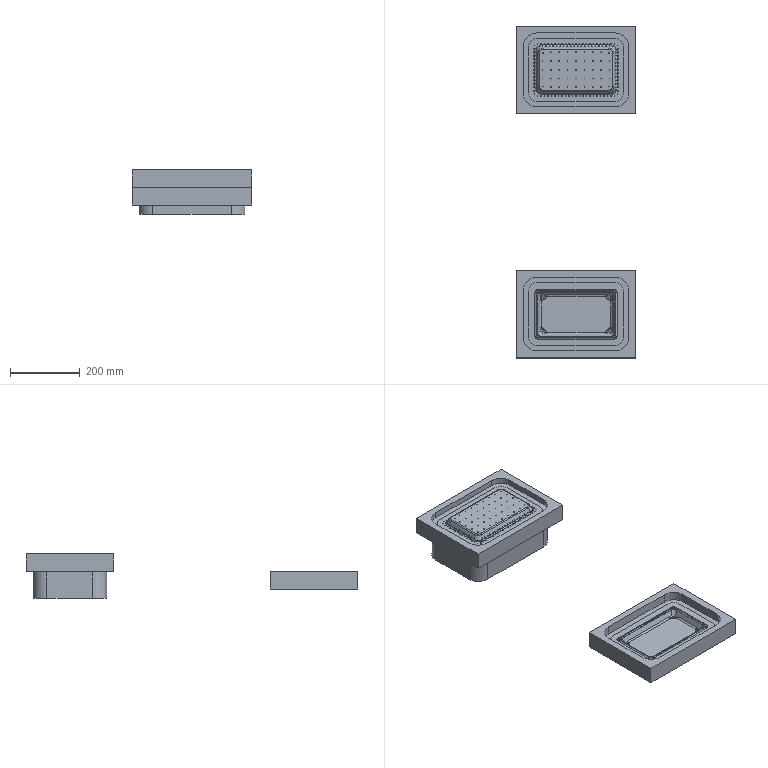NC program | NX | posted with a generic post | part box 343.99 x 952.259 x 127.368 mm
Lines 1 to 1066 of 51088:
N10 G17 G21 G94 G90
(CAVITY_MILL_3 , TOOL : D16R0.8)
N12 T00 M6
N14 G53
N16 G17 G0 G90 X90.744 Y252.89 S8000 M3 M8
N18 G43 Z200.5 H0
N20 Z51.5
N22 G94 G1 X64.131 Z50.105 F4000.
N24 X59.583
N26 G2 X27.89 Y284.583 R31.693
N28 G1 Y416.546
N30 G2 X59.583 Y448.24 R31.693
N32 G1 X284.407
N34 G2 X316.1 Y416.546 R31.693
N36 G1 Y284.583
N38 G2 X284.407 Y252.89 R31.693
N40 G1 X64.131
N42 Y262.97
N44 X59.583
N46 G2 X37.97 Y284.583 R21.613
N48 G1 Y416.546
N50 G2 X59.583 Y438.16 R21.613
N52 G1 X284.407
N54 G2 X306.02 Y416.546 R21.613
N56 G1 Y284.583
N58 G2 X284.407 Y262.97 R21.613
N60 G1 X64.131
N62 Y273.05
N64 X59.583
N66 G2 X48.05 Y284.583 R11.533
N68 G1 Y416.546
N70 G2 X59.583 Y428.08 R11.533
N72 G1 X68.679
N74 Y418.
N76 G3 X58.13 Y407.451 R21.562
N78 G1 Y416.546
N80 G2 X59.583 Y418. R1.453
N82 G1 X68.679
N84 X75.628 Y419.881
N86 G2 X77.71 Y419.982 R21.562
N88 G1 X266.28
N90 G2 X268.361 Y419.881 R21.562
N92 X268.712 Y420.88 R7.2
N94 G1 X75.278
N96 G2 X75.628 Y419.881 R7.2
N98 G1 X68.679 Y418.
N100 Y428.08
N102 X284.407
N104 G2 X295.94 Y416.546 R11.533
N106 G1 Y407.451
N108 X285.86
N110 G3 X275.311 Y418. R21.562
N112 G1 X284.407
N114 G2 X285.86 Y416.546 R1.453
N116 G1 Y407.451
N118 X287.742 Y400.501
N120 G2 X287.843 Y398.42 R21.562
N122 G1 Y302.71
N124 G2 X287.742 Y300.628 R21.562
N126 X288.74 Y300.278 R7.2
N128 G1 Y400.852
N130 G2 X287.742 Y400.501 R7.2
N132 G1 X285.86 Y407.451
N134 X295.94
N136 Y284.583
N138 G2 X284.407 Y273.05 R11.533
N140 G1 X275.311
N142 Y283.13
N144 G3 X285.86 Y293.679 R21.562
N146 G1 Y284.583
N148 G2 X284.407 Y283.13 R1.453
N150 G1 X275.311
N152 Y273.05
N154 X64.131
N156 Y283.13
N158 X59.583
N160 G2 X58.13 Y284.583 R1.453
N162 G1 Y293.679
N164 X56.248 Y300.628
N166 G2 X56.147 Y302.71 R21.562
N168 G1 Y398.42
N170 G2 X56.248 Y400.501 R21.562
N172 X55.25 Y400.852 R7.2
N174 G1 Y300.278
N176 G2 X56.248 Y300.628 R7.2
N178 G1 X58.13 Y293.679
N180 G3 X68.679 Y283.13 R21.562
N182 G1 X75.278 Y280.25
N184 X268.712
N186 G2 X268.361 Y281.248 R7.2
N188 X266.28 Y281.147 R21.562
N190 G1 X77.71
N192 G2 X75.628 Y281.248 R21.562
N194 X75.278 Y280.25 R7.2
N196 G1 X68.679 Y283.13
N198 X69.523 Y284.96
N200 G2 X58.163 Y302.71 R19.546
N202 G1 Y398.42
N204 G2 X77.71 Y417.966 R19.546
N206 G1 X266.28
N208 G2 X285.827 Y398.42 R19.546
N210 G1 Y302.71
N212 G2 X266.28 Y283.163 R19.546
N214 G1 X77.71
N216 G2 X69.523 Y284.96 R19.546
N218 G1 X68.679 Y283.13
N220 X64.131
N222 G3 X60.931 Y279.93 R3.2
N224 G1 Z51.105
N226 G0 Z53.5
N228 X90.744 Y253.
N230 Z51.105
N232 G1 X64.131 Z49.711
N234 X59.583
N236 G2 X28. Y284.583 R31.583
N238 G1 Y416.546
N240 G2 X59.583 Y448.129 R31.583
N242 G1 X284.407
N244 G2 X315.99 Y416.546 R31.583
N246 G1 Y284.583
N248 G2 X284.407 Y253. R31.583
N250 G1 X64.131
N252 Y263.08
N254 X59.583
N256 G2 X38.08 Y284.583 R21.503
N258 G1 Y416.546
N260 G2 X59.583 Y438.049 R21.503
N262 G1 X284.407
N264 G2 X305.91 Y416.546 R21.503
N266 G1 Y284.583
N268 G2 X284.407 Y263.08 R21.503
N270 G1 X64.131
N272 Y273.16
N274 X59.583
N276 G2 X48.16 Y284.583 R11.423
N278 G1 Y416.546
N280 G2 X59.583 Y427.969 R11.423
N282 G1 X66.85
N284 Y417.889
N286 G3 X58.24 Y409.279 R22.294
N288 G1 Y416.546
N290 G2 X59.583 Y417.889 R1.343
N292 G1 X66.85
N294 X73.622 Y420.335
N296 G2 X77.71 Y420.713 R22.294
N298 G1 X266.28
N300 G2 X270.368 Y420.335 R22.294
N302 X270.541 Y420.769 R7.2
N304 G1 X73.449
N306 G2 X73.622 Y420.335 R7.2
N308 G1 X66.85 Y417.889
N310 Y427.969
N312 X284.407
N314 G2 X295.83 Y416.546 R11.423
N316 G1 Y409.279
N318 X285.75
N320 G3 X277.14 Y417.889 R22.294
N322 G1 X284.407
N324 G2 X285.75 Y416.546 R1.343
N326 G1 Y409.279
N328 X288.196 Y402.507
N330 G2 X288.574 Y398.42 R22.294
N332 G1 Y302.71
N334 G2 X288.196 Y298.622 R22.294
N336 X288.63 Y298.449 R7.2
N338 G1 Y402.68
N340 G2 X288.196 Y402.507 R7.2
N342 G1 X285.75 Y409.279
N344 X295.83
N346 Y284.583
N348 G2 X284.407 Y273.16 R11.423
N350 G1 X277.14
N352 Y283.24
N354 G3 X285.75 Y291.85 R22.294
N356 G1 Y284.583
N358 G2 X284.407 Y283.24 R1.343
N360 G1 X277.14
N362 Y273.16
N364 X64.131
N366 Y283.24
N368 X59.583
N370 G2 X58.24 Y284.583 R1.343
N372 G1 Y291.85
N374 X55.794 Y298.622
N376 G2 X55.416 Y302.71 R22.294
N378 G1 Y398.42
N380 G2 X55.794 Y402.507 R22.294
N382 X55.36 Y402.68 R7.2
N384 G1 Y298.449
N386 G2 X55.794 Y298.622 R7.2
N388 G1 X58.24 Y291.85
N390 G3 X66.85 Y283.24 R22.294
N392 G1 X73.449 Y280.36
N394 X270.541
N396 G2 X270.368 Y280.794 R7.2
N398 X266.28 Y280.416 R22.294
N400 G1 X77.71
N402 G2 X73.622 Y280.794 R22.294
N404 X73.449 Y280.36 R7.2
N406 G1 X66.85 Y283.24
N408 X67.832 Y285.001
N410 G2 X57.432 Y302.71 R20.278
N412 G1 Y398.42
N414 G2 X77.71 Y418.697 R20.278
N416 G1 X266.28
N418 G2 X286.558 Y398.42 R20.278
N420 G1 Y302.71
N422 G2 X266.28 Y282.432 R20.278
N424 G1 X77.71
N426 G2 X67.832 Y285.001 R20.278
N428 G1 X66.85 Y283.24
N430 X64.131
N432 G3 X60.931 Y280.04 R3.2
N434 G1 Z50.711
N436 G0 Z53.105
N438 X90.744 Y253.
N440 Z50.711
N442 G1 X64.131 Z49.316
N444 X59.583
N446 G2 X28. Y284.583 R31.583
N448 G1 Y416.546
N450 G2 X59.583 Y448.129 R31.583
N452 G1 X284.407
N454 G2 X315.99 Y416.546 R31.583
N456 G1 Y284.583
N458 G2 X284.407 Y253. R31.583
N460 G1 X64.131
N462 Y263.08
N464 X59.583
N466 G2 X38.08 Y284.583 R21.503
N468 G1 Y416.546
N470 G2 X59.583 Y438.049 R21.503
N472 G1 X284.407
N474 G2 X305.91 Y416.546 R21.503
N476 G1 Y284.583
N478 G2 X284.407 Y263.08 R21.503
N480 G1 X64.131
N482 Y273.16
N484 X59.583
N486 G2 X48.16 Y284.583 R11.423
N488 G1 Y416.546
N490 G2 X59.583 Y427.969 R11.423
N492 G1 X65.82
N494 Y417.889
N496 G3 X58.24 Y410.309 R22.813
N498 G1 X55.408 Y403.454
N500 X58.24 Y410.309
N502 Y416.546
N504 G2 X59.583 Y417.889 R1.343
N506 G1 X65.82
N508 X72.675 Y420.722
N510 X65.82 Y417.889
N512 Y427.969
N514 X284.407
N516 G2 X295.83 Y416.546 R11.423
N518 G1 Y410.309
N520 X285.75
N522 G3 X278.17 Y417.889 R22.813
N524 G1 X271.314 Y420.722
N526 X278.17 Y417.889
N528 X284.407
N530 G2 X285.75 Y416.546 R1.343
N532 G1 Y410.309
N534 X288.582 Y403.454
N536 X285.75 Y410.309
N538 X295.83
N540 Y284.583
N542 G2 X284.407 Y273.16 R11.423
N544 G1 X278.17
N546 Y283.24
N548 G3 X285.75 Y290.82 R22.813
N550 G1 X288.582 Y297.675
N552 X285.75 Y290.82
N554 Y284.583
N556 G2 X284.407 Y283.24 R1.343
N558 G1 X278.17
N560 X271.314 Y280.408
N562 X278.17 Y283.24
N564 Y273.16
N566 X64.131
N568 Y283.24
N570 X59.583
N572 G2 X58.24 Y284.583 R1.343
N574 G1 Y290.82
N576 X55.408 Y297.675
N578 X58.24 Y290.82
N580 G3 X65.82 Y283.24 R22.813
N582 G1 X72.675 Y280.408
N584 X65.82 Y283.24
N586 X66.871 Y284.961
N588 G2 X56.913 Y302.71 R20.797
N590 G1 Y398.42
N592 G2 X77.71 Y419.217 R20.797
N594 G1 X266.28
N596 G2 X287.077 Y398.42 R20.797
N598 G1 Y302.71
N600 G2 X266.28 Y281.913 R20.797
N602 G1 X77.71
N604 G2 X66.871 Y284.961 R20.797
N606 G1 X65.82 Y283.24
N608 X64.131
N610 G3 X60.931 Y280.04 R3.2
N612 G1 Z50.316
N614 G0 Z52.711
N616 X90.744 Y253.
N618 Z50.316
N620 G1 X64.131 Z48.921
N622 X59.583
N624 G2 X28. Y284.583 R31.583
N626 G1 Y416.546
N628 G2 X59.583 Y448.129 R31.583
N630 G1 X284.407
N632 G2 X315.99 Y416.546 R31.583
N634 G1 Y284.583
N636 G2 X284.407 Y253. R31.583
N638 G1 X64.131
N640 Y263.08
N642 X59.583
N644 G2 X38.08 Y284.583 R21.503
N646 G1 Y416.546
N648 G2 X59.583 Y438.049 R21.503
N650 G1 X284.407
N652 G2 X305.91 Y416.546 R21.503
N654 G1 Y284.583
N656 G2 X284.407 Y263.08 R21.503
N658 G1 X64.131
N660 Y273.16
N662 X59.583
N664 G2 X48.16 Y284.583 R11.423
N666 G1 Y416.546
N668 G2 X59.583 Y427.969 R11.423
N670 G1 X65.066
N672 Y417.889
N674 G3 X58.24 Y411.063 R23.215
N676 G1 Y416.546
N678 G2 X59.583 Y417.889 R1.343
N680 G1 X65.066
N682 Y427.969
N684 X284.407
N686 G2 X295.83 Y416.546 R11.423
N688 G1 Y411.063
N690 X285.75
N692 G3 X278.924 Y417.889 R23.215
N694 G1 X284.407
N696 G2 X285.75 Y416.546 R1.343
N698 G1 Y411.063
N700 X295.83
N702 Y284.583
N704 G2 X284.407 Y273.16 R11.423
N706 G1 X278.924
N708 Y283.24
N710 G3 X285.75 Y290.066 R23.215
N712 G1 Y284.583
N714 G2 X284.407 Y283.24 R1.343
N716 G1 X278.924
N718 Y273.16
N720 X64.131
N722 Y283.24
N724 X59.583
N726 G2 X58.24 Y284.583 R1.343
N728 G1 Y290.066
N730 G3 X65.066 Y283.24 R23.215
N732 G1 X66.164 Y284.931
N734 G2 X56.511 Y302.71 R21.199
N736 G1 Y398.42
N738 G2 X77.71 Y419.619 R21.199
N740 G1 X266.28
N742 G2 X287.479 Y398.42 R21.199
N744 G1 Y302.71
N746 G2 X266.28 Y281.511 R21.199
N748 G1 X77.71
N750 G2 X66.164 Y284.931 R21.199
N752 G1 X65.066 Y283.24
N754 X64.131
N756 G3 X60.931 Y280.04 R3.2
N758 G1 Z49.921
N760 G0 Z52.316
N762 X90.744 Y253.
N764 Z49.921
N766 G1 X64.131 Z48.526
N768 X59.583
N770 G2 X28. Y284.583 R31.583
N772 G1 Y416.546
N774 G2 X59.583 Y448.129 R31.583
N776 G1 X284.407
N778 G2 X315.99 Y416.546 R31.583
N780 G1 Y284.583
N782 G2 X284.407 Y253. R31.583
N784 G1 X64.131
N786 Y263.08
N788 X59.583
N790 G2 X38.08 Y284.583 R21.503
N792 G1 Y416.546
N794 G2 X59.583 Y438.049 R21.503
N796 G1 X284.407
N798 G2 X305.91 Y416.546 R21.503
N800 G1 Y284.583
N802 G2 X284.407 Y263.08 R21.503
N804 G1 X64.131
N806 Y273.16
N808 X59.583
N810 G2 X48.16 Y284.583 R11.423
N812 G1 Y416.546
N814 G2 X59.583 Y427.969 R11.423
N816 G1 X64.473
N818 Y417.889
N820 G3 X58.24 Y411.664 R23.445
N822 G1 Y416.546
N824 G2 X59.583 Y417.889 R1.343
N826 G1 X64.473
N828 Y427.969
N830 X284.407
N832 G2 X295.83 Y416.546 R11.423
N834 G1 Y411.656
N836 X285.75
N838 G3 X279.52 Y417.889 R23.407
N840 G1 X284.407
N842 G2 X285.75 Y416.546 R1.343
N844 G1 Y411.656
N846 X295.83
N848 Y284.583
N850 G2 X284.407 Y273.16 R11.423
N852 G1 X279.516
N854 Y283.24
N856 G3 X285.75 Y289.465 R23.455
N858 G1 Y284.583
N860 G2 X284.407 Y283.24 R1.343
N862 G1 X279.516
N864 Y273.16
N866 X64.131
N868 Y283.24
N870 X59.583
N872 G2 X58.24 Y284.583 R1.343
N874 G1 Y289.474
N876 G3 X64.469 Y283.24 R23.41
N878 G1 X65.601 Y284.908
N880 G2 X56.274 Y301.15 R21.394
N882 G1 X56.22 Y302.128
N884 X56.196 Y302.678
N886 X56.19 Y302.71
N888 Y398.42
N890 G2 X59.41 Y409.765 R22.044
N892 X74.17 Y419.632 R21.429
N894 X77.71 Y419.939 R23.513
N896 G1 X266.28
N898 G2 X277.788 Y416.614 R21.987
N900 X287.716 Y399.98 R21.391
N902 G1 X287.769 Y399.001
N904 X287.8 Y398.42
N906 Y302.71
N908 G2 X284.58 Y291.365 R22.046
N910 X269.82 Y281.497 R21.439
N912 X266.28 Y281.19 R23.477
N914 G1 X77.71
N916 G2 X66.201 Y284.515 R21.994
N918 X65.601 Y284.908 R21.394
N920 G1 X64.469 Y283.24
N922 X64.131
N924 G3 X60.931 Y280.04 R3.2
N926 G1 Z49.526
N928 G0 Z51.921
N930 X90.744 Y253.
N932 Z49.526
N934 G1 X64.131 Z48.132
N936 X59.583
N938 G2 X28. Y284.583 R31.583
N940 G1 Y416.546
N942 G2 X59.583 Y448.129 R31.583
N944 G1 X284.407
N946 G2 X315.99 Y416.546 R31.583
N948 G1 Y284.583
N950 G2 X284.407 Y253. R31.583
N952 G1 X64.131
N954 Y263.08
N956 X59.583
N958 G2 X38.08 Y284.583 R21.503
N960 G1 Y416.546
N962 G2 X59.583 Y438.049 R21.503
N964 G1 X284.407
N966 G2 X305.91 Y416.546 R21.503
N968 G1 Y284.583
N970 G2 X284.407 Y263.08 R21.503
N972 G1 X64.131
N974 Y273.16
N976 X59.583
N978 G2 X48.16 Y284.583 R11.423
N980 G1 Y289.007
N982 X58.24
N984 G3 X64.018 Y283.24 R23.723
N986 G1 X59.583
N988 G2 X58.24 Y284.583 R1.343
N990 G1 Y289.007
N992 X48.16
N994 Y416.546
N996 G2 X59.583 Y427.969 R11.423
N998 G1 X63.997
N1000 Y417.889
N1002 G3 X58.24 Y412.108 R23.868
N1004 G1 Y416.546
N1006 G2 X59.583 Y417.889 R1.343
N1008 G1 X63.997
N1010 Y427.969
N1012 X284.407
N1014 G2 X295.83 Y416.546 R11.423
N1016 G1 Y412.126
N1018 X285.75
N1020 G3 X279.98 Y417.889 R23.635
N1022 G1 X284.407
N1024 G2 X285.75 Y416.546 R1.343
N1026 G1 Y412.126
N1028 X295.83
N1030 Y284.583
N1032 G2 X284.407 Y273.16 R11.423
N1034 G1 X279.986
N1036 Y283.24
N1038 G3 X285.75 Y289.009 R23.638
N1040 G1 X284.099 Y290.166
N1042 G2 X269.427 Y281.172 R21.622
N1044 X266.28 Y280.931 R24.654
N1046 G1 X77.71
N1048 G2 X75.176 Y281.097 R26.271
N1050 X55.931 Y302.663 R21.707
N1052 G1 Y398.42
N1054 G2 X65.366 Y416.387 R21.852
N1056 X76.599 Y420.142 R21.713
N1058 G1 X77.665 Y420.192
N1060 X77.71 Y420.198
N1062 X266.28
N1064 G2 X270.06 Y419.846 R24.794
N1066 X288.017 Y399.304 R21.619
N1068 G1 X288.046 Y398.506
N1070 X288.059 Y398.42
N1072 Y302.71
N1074 G2 X287.69 Y298.827 R24.449
N1076 X284.099 Y290.166 R21.622
N1078 G1 X285.75 Y289.009
N1080 Y284.583
N1082 G2 X284.407 Y283.24 R1.343
N1084 G1 X279.986
N1086 Y273.16
N1088 X64.131
N1090 G3 X60.931 Y269.96 R3.2
N1092 G1 Z49.132
N1094 G0 Z51.526
N1096 X90.744 Y253.
N1098 Z49.132
N1100 G1 X64.131 Z47.737
N1102 X59.583
N1104 G2 X28. Y284.583 R31.583
N1106 G1 Y416.546
N1108 G2 X59.583 Y448.129 R31.583
N1110 G1 X284.407
N1112 G2 X315.99 Y416.546 R31.583
N1114 G1 Y284.583
N1116 G2 X284.407 Y253. R31.583
N1118 G1 X64.131
N1120 Y263.08
N1122 X59.583
N1124 G2 X38.08 Y284.583 R21.503
N1126 G1 Y416.546
N1128 G2 X59.583 Y438.049 R21.503
N1130 G1 X284.407
N1132 G2 X305.91 Y416.546 R21.503
N1134 G1 Y284.583
N1136 G2 X284.407 Y263.08 R21.503
N1138 G1 X64.131
N1140 Y273.16
N1142 X59.583
N1144 G2 X48.16 Y284.583 R11.423
N1146 G1 Y288.618
N1148 X58.24
N1150 G3 X63.62 Y283.24 R23.915
N1152 G1 X59.583
N1154 G2 X58.24 Y284.583 R1.343
N1156 G1 Y288.618
N1158 X48.16
N1160 Y416.546
N1162 G2 X59.583 Y427.969 R11.423
N1164 G1 X63.618
N1166 Y417.889
N1168 G3 X58.24 Y412.502 R23.973
N1170 G1 Y416.546
N1172 G2 X59.583 Y417.889 R1.343
N1174 G1 X63.618
N1176 Y427.969
N1178 X284.407
N1180 G2 X295.83 Y416.546 R11.423
N1182 G1 Y412.525
N1184 X285.75
N1186 G3 X280.383 Y417.889 R23.775
N1188 G1 X284.407
N1190 G2 X285.75 Y416.546 R1.343
N1192 G1 Y412.525
N1194 X295.83
N1196 Y284.583
N1198 G2 X284.407 Y273.16 R11.423
N1200 G1 X280.382
N1202 Y283.24
N1204 G3 X285.75 Y288.611 R23.804
N1206 G1 X284.115 Y289.791
N1208 G2 X267.086 Y280.759 R21.788
N1210 G1 X266.885 Y280.753
N1212 X266.28 Y280.723
N1214 X77.71
N1216 G2 X70.257 Y282.004 R23.244
N1218 X55.723 Y302.71 R21.899
N1220 G1 Y398.42
N1222 G2 X66.883 Y417.593 R21.957
N1224 X77.71 Y420.406 R22.573
N1226 G1 X266.28
N1228 G2 X271.292 Y419.827 R23.36
N1230 X288.11 Y400.914 R21.759
N1232 G1 X288.21 Y399.98
N1234 X288.238 Y399.001
N1236 X288.264 Y398.512
N1238 X288.267 Y398.42
N1240 Y302.71
N1242 G2 X288.025 Y299.538 R25.683
N1244 X284.115 Y289.791 R21.788
N1246 G1 X285.75 Y288.611
N1248 Y284.583
N1250 G2 X284.407 Y283.24 R1.343
N1252 G1 X280.382
N1254 Y273.16
N1256 X64.131
N1258 G3 X60.931 Y269.96 R3.2
N1260 G1 Z48.737
N1262 G0 Z51.132
N1264 X90.744 Y253.
N1266 Z48.737
N1268 G1 X64.131 Z47.342
N1270 X59.583
N1272 G2 X28. Y284.583 R31.583
N1274 G1 Y416.546
N1276 G2 X59.583 Y448.129 R31.583
N1278 G1 X284.407
N1280 G2 X315.99 Y416.546 R31.583
N1282 G1 Y284.583
N1284 G2 X284.407 Y253. R31.583
N1286 G1 X64.131
N1288 Y263.08
N1290 X59.583
N1292 G2 X38.08 Y284.583 R21.503
N1294 G1 Y416.546
N1296 G2 X59.583 Y438.049 R21.503
N1298 G1 X284.407
N1300 G2 X305.91 Y416.546 R21.503
N1302 G1 Y284.583
N1304 G2 X284.407 Y263.08 R21.503
N1306 G1 X64.131
N1308 Y273.16
N1310 X59.583
N1312 G2 X48.16 Y284.583 R11.423
N1314 G1 Y288.243
N1316 X58.24
N1318 G3 X63.243 Y283.24 R24.008
N1320 G1 X59.583
N1322 G2 X58.24 Y284.583 R1.343
N1324 G1 Y288.243
N1326 X48.16
N1328 Y416.546
N1330 G2 X59.583 Y427.969 R11.423
N1332 G1 X63.243
N1334 Y417.889
N1336 G3 X58.24 Y412.887 R24.007
N1338 G1 Y416.546
N1340 G2 X59.583 Y417.889 R1.343
N1342 G1 X63.243
N1344 Y427.969
N1346 X284.407
N1348 G2 X295.83 Y416.546 R11.423
N1350 G1 Y412.886
N1352 X285.75
N1354 G3 X280.747 Y417.889 R24.008
N1356 G1 X284.407
N1358 G2 X285.75 Y416.546 R1.343
N1360 G1 Y412.886
N1362 X295.83
N1364 Y284.583
N1366 G2 X284.407 Y273.16 R11.423
N1368 G1 X280.745
N1370 Y283.24
N1372 G3 X285.75 Y288.245 R24.011
N1374 G1 X284.13 Y289.445
N1376 G2 X266.371 Y280.541 R21.995
N1378 G1 X77.619
N1380 G2 X55.541 Y302.619 R21.992
N1382 G1 Y398.51
N1384 G2 X77.619 Y420.589 R21.991
N1386 G1 X266.371
N1388 G2 X288.449 Y398.51 R21.992
N1390 G1 Y302.619
N1392 G2 X284.13 Y289.445 R21.995
N1394 G1 X285.75 Y288.245
N1396 Y284.583
N1398 G2 X284.407 Y283.24 R1.343
N1400 G1 X280.745
N1402 Y273.16
N1404 X64.131
N1406 G3 X60.931 Y269.96 R3.2
N1408 G1 Z48.342
N1410 G0 Z50.737
N1412 X90.744 Y253.
N1414 Z48.342
N1416 G1 X64.131 Z46.948
N1418 X59.583
N1420 G2 X28. Y284.583 R31.583
N1422 G1 Y416.546
N1424 G2 X59.583 Y448.129 R31.583
N1426 G1 X284.407
N1428 G2 X315.99 Y416.546 R31.583
N1430 G1 Y284.583
N1432 G2 X284.407 Y253. R31.583
N1434 G1 X64.131
N1436 Y263.08
N1438 X59.583
N1440 G2 X38.08 Y284.583 R21.503
N1442 G1 Y416.546
N1444 G2 X59.583 Y438.049 R21.503
N1446 G1 X284.407
N1448 G2 X305.91 Y416.546 R21.503
N1450 G1 Y284.583
N1452 G2 X284.407 Y263.08 R21.503
N1454 G1 X64.131
N1456 Y273.16
N1458 X59.583
N1460 G2 X48.16 Y284.583 R11.423
N1462 G1 Y287.878
N1464 X58.24
N1466 G3 X62.878 Y283.24 R24.098
N1468 G1 X59.583
N1470 G2 X58.24 Y284.583 R1.343
N1472 G1 Y287.878
N1474 X48.16
N1476 Y416.546
N1478 G2 X59.583 Y427.969 R11.423
N1480 G1 X62.877
N1482 Y417.889
N1484 G3 X58.24 Y413.252 R24.098
N1486 G1 Y416.546
N1488 G2 X59.583 Y417.889 R1.343
N1490 G1 X62.877
N1492 Y427.969
N1494 X284.407
N1496 G2 X295.83 Y416.546 R11.423
N1498 G1 Y413.251
N1500 X285.75
N1502 G3 X281.111 Y417.889 R24.1
N1504 G1 X284.407
N1506 G2 X285.75 Y416.546 R1.343
N1508 G1 Y413.251
N1510 X295.83
N1512 Y284.583
N1514 G2 X284.407 Y273.16 R11.423
N1516 G1 X281.111
N1518 Y283.24
N1520 G3 X285.75 Y287.879 R24.101
N1522 G1 X284.144 Y289.097
N1524 G2 X266.467 Y280.358 R22.085
N1526 G1 X77.523
N1528 G2 X55.358 Y302.523 R22.082
N1530 G1 Y398.606
N1532 G2 X77.523 Y420.771 R22.082
N1534 G1 X266.467
N1536 G2 X288.632 Y398.606 R22.084
N1538 G1 Y302.523
N1540 G2 X284.144 Y289.097 R22.085
N1542 G1 X285.75 Y287.879
N1544 Y284.583
N1546 G2 X284.407 Y283.24 R1.343
N1548 G1 X281.111
N1550 Y273.16
N1552 X64.131
N1554 G3 X60.931 Y269.96 R3.2
N1556 G1 Z47.948
N1558 G0 Z50.342
N1560 X90.744 Y253.
N1562 Z47.948
N1564 G1 X64.131 Z46.553
N1566 X59.583
N1568 G2 X28. Y284.583 R31.583
N1570 G1 Y416.546
N1572 G2 X59.583 Y448.129 R31.583
N1574 G1 X284.407
N1576 G2 X315.99 Y416.546 R31.583
N1578 G1 Y284.583
N1580 G2 X284.407 Y253. R31.583
N1582 G1 X64.131
N1584 Y263.08
N1586 X59.583
N1588 G2 X38.08 Y284.583 R21.503
N1590 G1 Y416.546
N1592 G2 X59.583 Y438.049 R21.503
N1594 G1 X284.407
N1596 G2 X305.91 Y416.546 R21.503
N1598 G1 Y284.583
N1600 G2 X284.407 Y263.08 R21.503
N1602 G1 X64.131
N1604 Y273.16
N1606 X59.583
N1608 G2 X48.16 Y284.583 R11.423
N1610 G1 Y287.514
N1612 X58.24
N1614 G3 X62.514 Y283.24 R24.183
N1616 G1 X59.583
N1618 G2 X58.24 Y284.583 R1.343
N1620 G1 Y287.514
N1622 X48.16
N1624 Y416.546
N1626 G2 X59.583 Y427.969 R11.423
N1628 G1 X62.512
N1630 Y417.889
N1632 G3 X58.24 Y413.617 R24.181
N1634 G1 Y416.546
N1636 G2 X59.583 Y417.889 R1.343
N1638 G1 X62.512
N1640 Y427.969
N1642 X284.407
N1644 G2 X295.83 Y416.546 R11.423
N1646 G1 Y413.616
N1648 X285.75
N1650 G3 X281.476 Y417.889 R24.184
N1652 G1 X284.407
N1654 G2 X285.75 Y416.546 R1.343
N1656 G1 Y413.616
N1658 X295.83
N1660 Y284.583
N1662 G2 X284.407 Y273.16 R11.423
N1664 G1 X281.478
N1666 Y283.24
N1668 G3 X285.75 Y287.512 R24.181
N1670 G1 X284.157 Y288.748
N1672 G2 X266.563 Y280.176 R22.165
N1674 G1 X77.427
N1676 G2 X55.176 Y302.427 R22.167
N1678 G1 Y398.703
N1680 G2 X77.427 Y420.954 R22.165
N1682 G1 X266.563
N1684 G2 X288.814 Y398.703 R22.168
N1686 G1 Y302.427
N1688 G2 X284.157 Y288.748 R22.165
N1690 G1 X285.75 Y287.512
N1692 Y284.583
N1694 G2 X284.407 Y283.24 R1.343
N1696 G1 X281.478
N1698 Y273.16
N1700 X64.131
N1702 G3 X60.931 Y269.96 R3.2
N1704 G1 Z47.553
N1706 G0 Z49.948
N1708 X90.744 Y253.
N1710 Z47.553
N1712 G1 X64.131 Z46.158
N1714 X59.583
N1716 G2 X28. Y284.583 R31.583
N1718 G1 Y416.546
N1720 G2 X59.583 Y448.129 R31.583
N1722 G1 X284.407
N1724 G2 X315.99 Y416.546 R31.583
N1726 G1 Y284.583
N1728 G2 X284.407 Y253. R31.583
N1730 G1 X64.131
N1732 Y263.08
N1734 X59.583
N1736 G2 X38.08 Y284.583 R21.503
N1738 G1 Y416.546
N1740 G2 X59.583 Y438.049 R21.503
N1742 G1 X284.407
N1744 G2 X305.91 Y416.546 R21.503
N1746 G1 Y284.583
N1748 G2 X284.407 Y263.08 R21.503
N1750 G1 X64.131
N1752 Y273.16
N1754 X59.583
N1756 G2 X48.16 Y284.583 R11.423
N1758 G1 Y287.156
N1760 X58.24
N1762 G3 X62.156 Y283.24 R24.271
N1764 G1 X59.583
N1766 G2 X58.24 Y284.583 R1.343
N1768 G1 Y287.156
N1770 X48.16
N1772 Y416.546
N1774 G2 X59.583 Y427.969 R11.423
N1776 G1 X62.151
N1778 Y417.889
N1780 G3 X58.24 Y413.978 R24.264
N1782 G1 Y416.546
N1784 G2 X59.583 Y417.889 R1.343
N1786 G1 X62.151
N1788 Y427.969
N1790 X284.407
N1792 G2 X295.83 Y416.546 R11.423
N1794 G1 Y413.976
N1796 X285.75
N1798 G3 X281.836 Y417.889 R24.267
N1800 G1 X284.407
N1802 G2 X285.75 Y416.546 R1.343
N1804 G1 Y413.976
N1806 X295.83
N1808 Y284.583
N1810 G2 X284.407 Y273.16 R11.423
N1812 G1 X281.838
N1814 Y283.24
N1816 G3 X285.75 Y287.152 R24.265
N1818 G1 X284.171 Y288.406
N1820 G2 X266.659 Y279.993 R22.249
N1822 G1 X77.331
N1824 G2 X54.993 Y302.331 R22.255
N1826 G1 Y398.799
N1828 G2 X77.331 Y421.136 R22.248
N1830 G1 X266.659
N1832 G2 X288.997 Y398.799 R22.251
N1834 G1 Y302.331
N1836 G2 X284.171 Y288.406 R22.249
N1838 G1 X285.75 Y287.152
N1840 Y284.583
N1842 G2 X284.407 Y283.24 R1.343
N1844 G1 X281.838
N1846 Y273.16
N1848 X64.131
N1850 G3 X60.931 Y269.96 R3.2
N1852 G1 Z47.158
N1854 G0 Z49.553
N1856 X90.744 Y253.
N1858 Z47.158
N1860 G1 X64.131 Z45.763
N1862 X59.583
N1864 G2 X28. Y284.583 R31.583
N1866 G1 Y416.546
N1868 G2 X59.583 Y448.129 R31.583
N1870 G1 X284.407
N1872 G2 X315.99 Y416.546 R31.583
N1874 G1 Y284.583
N1876 G2 X284.407 Y253. R31.583
N1878 G1 X64.131
N1880 Y263.08
N1882 X59.583
N1884 G2 X38.08 Y284.583 R21.503
N1886 G1 Y416.546
N1888 G2 X59.583 Y438.049 R21.503
N1890 G1 X284.407
N1892 G2 X305.91 Y416.546 R21.503
N1894 G1 Y284.583
N1896 G2 X284.407 Y263.08 R21.503
N1898 G1 X64.131
N1900 Y273.16
N1902 X59.583
N1904 G2 X48.16 Y284.583 R11.423
N1906 G1 Y286.803
N1908 X58.24
N1910 G3 X61.803 Y283.24 R24.359
N1912 G1 X59.583
N1914 G2 X58.24 Y284.583 R1.343
N1916 G1 Y286.803
N1918 X48.16
N1920 Y416.546
N1922 G2 X59.583 Y427.969 R11.423
N1924 G1 X61.797
N1926 Y417.889
N1928 G3 X58.24 Y414.332 R24.35
N1930 G1 Y416.546
N1932 G2 X59.583 Y417.889 R1.343
N1934 G1 X61.797
N1936 Y427.969
N1938 X284.407
N1940 G2 X295.83 Y416.546 R11.423
N1942 G1 Y414.333
N1944 X285.75
N1946 G3 X282.193 Y417.889 R24.349
N1948 G1 X284.407
N1950 G2 X285.75 Y416.546 R1.343
N1952 G1 Y414.333
N1954 X295.83
N1956 Y284.583
N1958 G2 X284.407 Y273.16 R11.423
N1960 G1 X282.19
N1962 Y283.24
N1964 G3 X285.75 Y286.8 R24.354
N1966 G1 X284.185 Y288.071
N1968 G2 X266.756 Y279.811 R22.338
N1970 G1 X77.234
N1972 G2 X54.811 Y302.234 R22.343
N1974 G1 Y398.895
N1976 G2 X77.234 Y421.318 R22.334
N1978 G1 X266.756
N1980 G2 X289.179 Y398.895 R22.333
N1982 G1 Y302.234
N1984 G2 X284.185 Y288.071 R22.338
N1986 G1 X285.75 Y286.8
N1988 Y284.583
N1990 G2 X284.407 Y283.24 R1.343
N1992 G1 X282.19
N1994 Y273.16
N1996 X64.131
N1998 G3 X60.931 Y269.96 R3.2
N2000 G1 Z46.763
N2002 G0 Z49.158
N2004 X90.744 Y253.
N2006 Z46.763
N2008 G1 X64.131 Z45.369
N2010 X59.583
N2012 G2 X28. Y284.583 R31.583
N2014 G1 Y416.546
N2016 G2 X59.583 Y448.129 R31.583
N2018 G1 X284.407
N2020 G2 X315.99 Y416.546 R31.583
N2022 G1 Y284.583
N2024 G2 X284.407 Y253. R31.583
N2026 G1 X64.131
N2028 Y263.08
N2030 X59.583
N2032 G2 X38.08 Y284.583 R21.503
N2034 G1 Y416.546
N2036 G2 X59.583 Y438.049 R21.503
N2038 G1 X284.407
N2040 G2 X305.91 Y416.546 R21.503
N2042 G1 Y284.583
N2044 G2 X284.407 Y263.08 R21.503
N2046 G1 X64.131
N2048 Y273.16
N2050 X59.583
N2052 G2 X48.16 Y284.583 R11.423
N2054 G1 Y286.454
N2056 X58.24
N2058 G3 X61.454 Y283.24 R24.446
N2060 G1 X59.583
N2062 G2 X58.24 Y284.583 R1.343
N2064 G1 Y286.454
N2066 X48.16
N2068 Y416.546
N2070 G2 X59.583 Y427.969 R11.423
N2072 G1 X61.451
N2074 Y417.889
N2076 G3 X58.24 Y414.679 R24.44
N2078 G1 Y416.546
N2080 G2 X59.583 Y417.889 R1.343
N2082 G1 X61.451
N2084 Y427.969
N2086 X284.407
N2088 G2 X295.83 Y416.546 R11.423
N2090 G1 Y414.675
N2092 X285.75
N2094 G3 X282.536 Y417.889 R24.445
N2096 G1 X284.407
N2098 G2 X285.75 Y416.546 R1.343
N2100 G1 Y414.675
N2102 X295.83
N2104 Y284.583
N2106 G2 X284.407 Y273.16 R11.423
N2108 G1 X282.541
N2110 Y283.24
N2112 G3 X285.75 Y286.449 R24.438
N2114 G1 X284.198 Y287.736
N2116 G2 X266.852 Y279.628 R22.422
N2118 G1 X77.138
N2120 G2 X54.628 Y302.138 R22.43
N2122 G1 Y398.991
N2124 G2 X77.138 Y421.501 R22.424
N2126 G1 X266.852
N2128 G2 X289.362 Y398.991 R22.429
N2130 G1 Y302.138